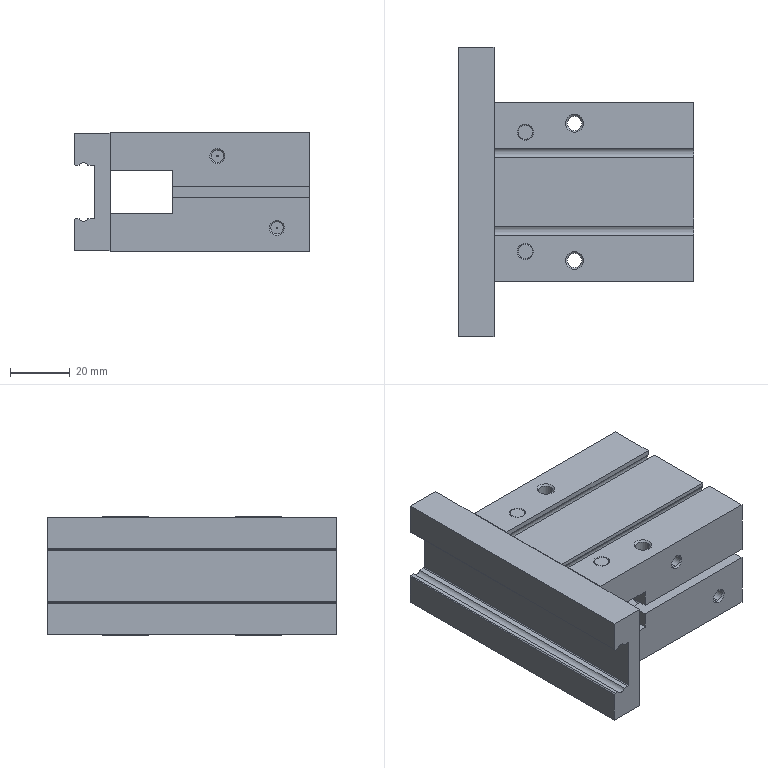Part | SolidWorks | features BaseBody 1 | 1 solid | 177 faces | box 79 x 97 x 40 mm | volume 159710 mm3 | plane 78 | cylinder 53 | cone 46 | commonest cylinder face diameters 4.917 x16 6.02 x8 0.4 x6 4.2 x6 0.5 x4 4.134 x4